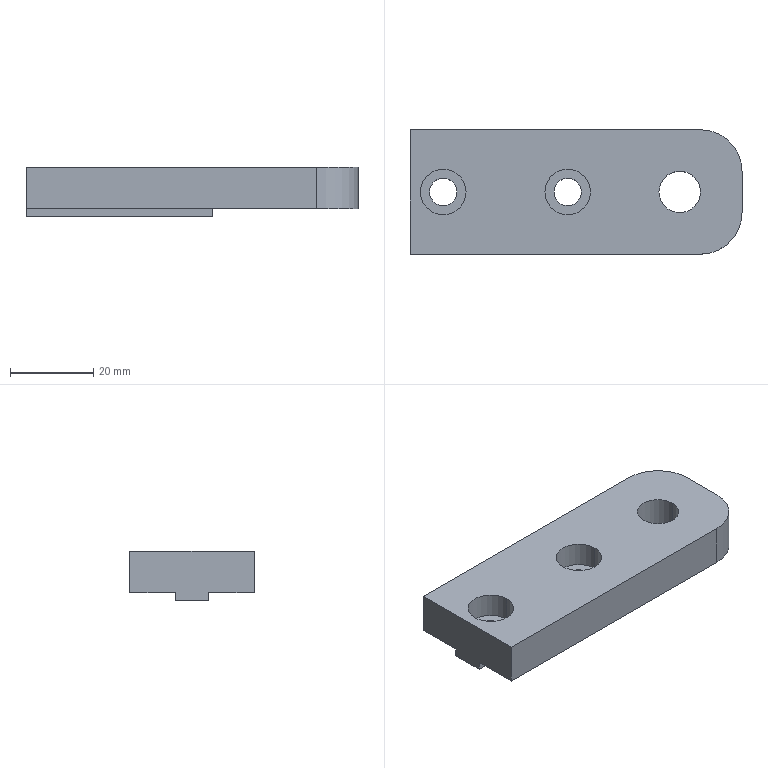Part | STEP file | 11-XSS10811 | 1 solid | 24 faces | box 80 x 30 x 12 mm | volume 21954 mm3 | cylinder 12 | plane 12 | commonest cylinder face diameters 6.6 x4 11 x4 10 x2 20 x2
STEP:
#1=CARTESIAN_POINT('',(-7.5,0.,4.));
#2=VERTEX_POINT('',#1);
#3=CARTESIAN_POINT('',(3.5,0.,4.));
#4=VERTEX_POINT('',#3);
#5=CARTESIAN_POINT('',(-2.,0.,4.));
#6=DIRECTION('',(0.,0.,1.));
#7=DIRECTION('',(1.,0.,0.));
#8=AXIS2_PLACEMENT_3D('',#5,#6,#7);
#9=CIRCLE('',#8,5.5);
#10=EDGE_CURVE('',#2,#4,#9,.T.);
#11=ORIENTED_EDGE('',*,*,#10,.F.);
#12=CARTESIAN_POINT('',(-7.5,0.,10.));
#13=VERTEX_POINT('',#12);
#14=CARTESIAN_POINT('',(-7.5,0.,10.));
#15=DIRECTION('',(0.,0.,1.));
#16=VECTOR('',#15,1000.);
#17=LINE('',#14,#16);
#18=EDGE_CURVE('',#2,#13,#17,.T.);
#19=ORIENTED_EDGE('',*,*,#18,.T.);
#20=CARTESIAN_POINT('',(3.5,0.,10.));
#21=VERTEX_POINT('',#20);
#22=CARTESIAN_POINT('',(-2.,0.,10.));
#23=DIRECTION('',(0.,0.,1.));
#24=DIRECTION('',(1.,0.,0.));
#25=AXIS2_PLACEMENT_3D('',#22,#23,#24);
#26=CIRCLE('',#25,5.5);
#27=EDGE_CURVE('',#13,#21,#26,.T.);
#28=ORIENTED_EDGE('',*,*,#27,.T.);
#29=CARTESIAN_POINT('',(3.5,0.,10.));
#30=DIRECTION('',(0.,0.,1.));
#31=VECTOR('',#30,1000.);
#32=LINE('',#29,#31);
#33=EDGE_CURVE('',#4,#21,#32,.T.);
#34=ORIENTED_EDGE('',*,*,#33,.F.);
#35=EDGE_LOOP('',(#11,#19,#28,#34));
#36=FACE_OUTER_BOUND('',#35,.T.);
#37=CARTESIAN_POINT('',(-2.,0.,10.));
#38=DIRECTION('',(0.,0.,1.));
#39=DIRECTION('',(1.,0.,0.));
#40=AXIS2_PLACEMENT_3D('',#37,#38,#39);
#41=CYLINDRICAL_SURFACE('',#40,5.5);
#42=ADVANCED_FACE('',(#36),#41,.F.);
#43=CARTESIAN_POINT('',(-5.3,0.,-2.));
#44=VERTEX_POINT('',#43);
#45=CARTESIAN_POINT('',(1.3,0.,-2.));
#46=VERTEX_POINT('',#45);
#47=CARTESIAN_POINT('',(-2.,0.,-2.));
#48=DIRECTION('',(0.,0.,1.));
#49=DIRECTION('',(1.,0.,0.));
#50=AXIS2_PLACEMENT_3D('',#47,#48,#49);
#51=CIRCLE('',#50,3.3);
#52=EDGE_CURVE('',#44,#46,#51,.T.);
#53=ORIENTED_EDGE('',*,*,#52,.F.);
#54=CARTESIAN_POINT('',(-5.3,0.,4.));
#55=VERTEX_POINT('',#54);
#56=CARTESIAN_POINT('',(-5.3,0.,10.));
#57=DIRECTION('',(0.,0.,1.));
#58=VECTOR('',#57,1000.);
#59=LINE('',#56,#58);
#60=EDGE_CURVE('',#44,#55,#59,.T.);
#61=ORIENTED_EDGE('',*,*,#60,.T.);
#62=CARTESIAN_POINT('',(1.3,0.,4.));
#63=VERTEX_POINT('',#62);
#64=CARTESIAN_POINT('',(-2.,0.,4.));
#65=DIRECTION('',(0.,0.,1.));
#66=DIRECTION('',(1.,0.,0.));
#67=AXIS2_PLACEMENT_3D('',#64,#65,#66);
#68=CIRCLE('',#67,3.3);
#69=EDGE_CURVE('',#55,#63,#68,.T.);
#70=ORIENTED_EDGE('',*,*,#69,.T.);
#71=CARTESIAN_POINT('',(1.3,0.,10.));
#72=DIRECTION('',(0.,0.,1.));
#73=VECTOR('',#72,1000.);
#74=LINE('',#71,#73);
#75=EDGE_CURVE('',#46,#63,#74,.T.);
#76=ORIENTED_EDGE('',*,*,#75,.F.);
#77=EDGE_LOOP('',(#53,#61,#70,#76));
#78=FACE_OUTER_BOUND('',#77,.T.);
#79=CARTESIAN_POINT('',(-2.,0.,10.));
#80=DIRECTION('',(0.,0.,1.));
#81=DIRECTION('',(1.,0.,0.));
#82=AXIS2_PLACEMENT_3D('',#79,#80,#81);
#83=CYLINDRICAL_SURFACE('',#82,3.3);
#84=ADVANCED_FACE('',(#78),#83,.F.);
#85=CARTESIAN_POINT('',(-37.5,0.,4.));
#86=VERTEX_POINT('',#85);
#87=CARTESIAN_POINT('',(-26.5,0.,4.));
#88=VERTEX_POINT('',#87);
#89=CARTESIAN_POINT('',(-32.,0.,4.));
#90=DIRECTION('',(0.,0.,1.));
#91=DIRECTION('',(1.,0.,0.));
#92=AXIS2_PLACEMENT_3D('',#89,#90,#91);
#93=CIRCLE('',#92,5.5);
#94=EDGE_CURVE('',#86,#88,#93,.T.);
#95=ORIENTED_EDGE('',*,*,#94,.F.);
#96=CARTESIAN_POINT('',(-37.5,0.,10.));
#97=VERTEX_POINT('',#96);
#98=CARTESIAN_POINT('',(-37.5,0.,10.));
#99=DIRECTION('',(0.,0.,1.));
#100=VECTOR('',#99,1000.);
#101=LINE('',#98,#100);
#102=EDGE_CURVE('',#86,#97,#101,.T.);
#103=ORIENTED_EDGE('',*,*,#102,.T.);
#104=CARTESIAN_POINT('',(-26.5,0.,10.));
#105=VERTEX_POINT('',#104);
#106=CARTESIAN_POINT('',(-32.,0.,10.));
#107=DIRECTION('',(0.,0.,1.));
#108=DIRECTION('',(1.,0.,0.));
#109=AXIS2_PLACEMENT_3D('',#106,#107,#108);
#110=CIRCLE('',#109,5.5);
#111=EDGE_CURVE('',#97,#105,#110,.T.);
#112=ORIENTED_EDGE('',*,*,#111,.T.);
#113=CARTESIAN_POINT('',(-26.5,0.,10.));
#114=DIRECTION('',(0.,0.,1.));
#115=VECTOR('',#114,1000.);
#116=LINE('',#113,#115);
#117=EDGE_CURVE('',#88,#105,#116,.T.);
#118=ORIENTED_EDGE('',*,*,#117,.F.);
#119=EDGE_LOOP('',(#95,#103,#112,#118));
#120=FACE_OUTER_BOUND('',#119,.T.);
#121=CARTESIAN_POINT('',(-32.,0.,10.));
#122=DIRECTION('',(0.,0.,1.));
#123=DIRECTION('',(1.,0.,0.));
#124=AXIS2_PLACEMENT_3D('',#121,#122,#123);
#125=CYLINDRICAL_SURFACE('',#124,5.5);
#126=ADVANCED_FACE('',(#120),#125,.F.);
#127=CARTESIAN_POINT('',(-35.3,0.,-2.));
#128=VERTEX_POINT('',#127);
#129=CARTESIAN_POINT('',(-28.7,0.,-2.));
#130=VERTEX_POINT('',#129);
#131=CARTESIAN_POINT('',(-32.,0.,-2.));
#132=DIRECTION('',(0.,0.,1.));
#133=DIRECTION('',(1.,0.,0.));
#134=AXIS2_PLACEMENT_3D('',#131,#132,#133);
#135=CIRCLE('',#134,3.3);
#136=EDGE_CURVE('',#128,#130,#135,.T.);
#137=ORIENTED_EDGE('',*,*,#136,.F.);
#138=CARTESIAN_POINT('',(-35.3,0.,4.));
#139=VERTEX_POINT('',#138);
#140=CARTESIAN_POINT('',(-35.3,0.,10.));
#141=DIRECTION('',(0.,0.,1.));
#142=VECTOR('',#141,1000.);
#143=LINE('',#140,#142);
#144=EDGE_CURVE('',#128,#139,#143,.T.);
#145=ORIENTED_EDGE('',*,*,#144,.T.);
#146=CARTESIAN_POINT('',(-28.7,0.,4.));
#147=VERTEX_POINT('',#146);
#148=CARTESIAN_POINT('',(-32.,0.,4.));
#149=DIRECTION('',(0.,0.,1.));
#150=DIRECTION('',(1.,0.,0.));
#151=AXIS2_PLACEMENT_3D('',#148,#149,#150);
#152=CIRCLE('',#151,3.3);
#153=EDGE_CURVE('',#139,#147,#152,.T.);
#154=ORIENTED_EDGE('',*,*,#153,.T.);
#155=CARTESIAN_POINT('',(-28.7,0.,10.));
#156=DIRECTION('',(0.,0.,1.));
#157=VECTOR('',#156,1000.);
#158=LINE('',#155,#157);
#159=EDGE_CURVE('',#130,#147,#158,.T.);
#160=ORIENTED_EDGE('',*,*,#159,.F.);
#161=EDGE_LOOP('',(#137,#145,#154,#160));
#162=FACE_OUTER_BOUND('',#161,.T.);
#163=CARTESIAN_POINT('',(-32.,0.,10.));
#164=DIRECTION('',(0.,0.,1.));
#165=DIRECTION('',(1.,0.,0.));
#166=AXIS2_PLACEMENT_3D('',#163,#164,#165);
#167=CYLINDRICAL_SURFACE('',#166,3.3);
#168=ADVANCED_FACE('',(#162),#167,.F.);
#169=CARTESIAN_POINT('',(20.,0.,0.));
#170=VERTEX_POINT('',#169);
#171=CARTESIAN_POINT('',(30.,0.,0.));
#172=VERTEX_POINT('',#171);
#173=CARTESIAN_POINT('',(25.,0.,0.));
#174=DIRECTION('',(0.,0.,1.));
#175=DIRECTION('',(1.,0.,0.));
#176=AXIS2_PLACEMENT_3D('',#173,#174,#175);
#177=CIRCLE('',#176,5.);
#178=EDGE_CURVE('',#170,#172,#177,.T.);
#179=ORIENTED_EDGE('',*,*,#178,.F.);
#180=CARTESIAN_POINT('',(20.,0.,10.));
#181=VERTEX_POINT('',#180);
#182=CARTESIAN_POINT('',(20.,0.,0.));
#183=DIRECTION('',(0.,0.,1.));
#184=VECTOR('',#183,1000.);
#185=LINE('',#182,#184);
#186=EDGE_CURVE('',#170,#181,#185,.T.);
#187=ORIENTED_EDGE('',*,*,#186,.T.);
#188=CARTESIAN_POINT('',(30.,0.,10.));
#189=VERTEX_POINT('',#188);
#190=CARTESIAN_POINT('',(25.,0.,10.));
#191=DIRECTION('',(0.,0.,1.));
#192=DIRECTION('',(1.,0.,0.));
#193=AXIS2_PLACEMENT_3D('',#190,#191,#192);
#194=CIRCLE('',#193,5.);
#195=EDGE_CURVE('',#181,#189,#194,.T.);
#196=ORIENTED_EDGE('',*,*,#195,.T.);
#197=CARTESIAN_POINT('',(30.,0.,0.));
#198=DIRECTION('',(0.,0.,1.));
#199=VECTOR('',#198,1000.);
#200=LINE('',#197,#199);
#201=EDGE_CURVE('',#172,#189,#200,.T.);
#202=ORIENTED_EDGE('',*,*,#201,.F.);
#203=EDGE_LOOP('',(#179,#187,#196,#202));
#204=FACE_OUTER_BOUND('',#203,.T.);
#205=CARTESIAN_POINT('',(25.,0.,0.));
#206=DIRECTION('',(0.,0.,1.));
#207=DIRECTION('',(1.,0.,0.));
#208=AXIS2_PLACEMENT_3D('',#205,#206,#207);
#209=CYLINDRICAL_SURFACE('',#208,5.);
#210=ADVANCED_FACE('',(#204),#209,.F.);
#211=CARTESIAN_POINT('',(25.,0.,0.));
#212=DIRECTION('',(0.,0.,1.));
#213=DIRECTION('',(1.,0.,0.));
#214=AXIS2_PLACEMENT_3D('',#211,#212,#213);
#215=CIRCLE('',#214,5.);
#216=EDGE_CURVE('',#172,#170,#215,.T.);
#217=ORIENTED_EDGE('',*,*,#216,.T.);
#218=ORIENTED_EDGE('',*,*,#178,.T.);
#219=EDGE_LOOP('',(#217,#218));
#220=FACE_BOUND('',#219,.T.);
#221=CARTESIAN_POINT('',(5.,-4.,0.));
#222=VERTEX_POINT('',#221);
#223=CARTESIAN_POINT('',(-40.,-4.,0.));
#224=VERTEX_POINT('',#223);
#225=CARTESIAN_POINT('',(-40.,-4.,0.));
#226=DIRECTION('',(-1.,0.,0.));
#227=VECTOR('',#226,1000.);
#228=LINE('',#225,#227);
#229=EDGE_CURVE('',#222,#224,#228,.T.);
#230=ORIENTED_EDGE('',*,*,#229,.F.);
#231=CARTESIAN_POINT('',(5.,4.,0.));
#232=VERTEX_POINT('',#231);
#233=CARTESIAN_POINT('',(5.,4.,0.));
#234=DIRECTION('',(0.,-1.,0.));
#235=VECTOR('',#234,1000.);
#236=LINE('',#233,#235);
#237=EDGE_CURVE('',#232,#222,#236,.T.);
#238=ORIENTED_EDGE('',*,*,#237,.F.);
#239=CARTESIAN_POINT('',(-40.,4.,0.));
#240=VERTEX_POINT('',#239);
#241=CARTESIAN_POINT('',(-40.,4.,0.));
#242=DIRECTION('',(1.,0.,0.));
#243=VECTOR('',#242,1000.);
#244=LINE('',#241,#243);
#245=EDGE_CURVE('',#240,#232,#244,.T.);
#246=ORIENTED_EDGE('',*,*,#245,.F.);
#247=CARTESIAN_POINT('',(-40.,15.,0.));
#248=VERTEX_POINT('',#247);
#249=CARTESIAN_POINT('',(-40.,15.,0.));
#250=DIRECTION('',(0.,-1.,0.));
#251=VECTOR('',#250,1000.);
#252=LINE('',#249,#251);
#253=EDGE_CURVE('',#248,#240,#252,.T.);
#254=ORIENTED_EDGE('',*,*,#253,.F.);
#255=CARTESIAN_POINT('',(30.,15.,0.));
#256=VERTEX_POINT('',#255);
#257=CARTESIAN_POINT('',(-40.,15.,0.));
#258=DIRECTION('',(-1.,0.,0.));
#259=VECTOR('',#258,1000.);
#260=LINE('',#257,#259);
#261=EDGE_CURVE('',#256,#248,#260,.T.);
#262=ORIENTED_EDGE('',*,*,#261,.F.);
#263=CARTESIAN_POINT('',(40.,5.,0.));
#264=VERTEX_POINT('',#263);
#265=CARTESIAN_POINT('',(30.,5.,0.));
#266=DIRECTION('',(0.,0.,-1.));
#267=DIRECTION('',(1.,0.,0.));
#268=AXIS2_PLACEMENT_3D('',#265,#266,#267);
#269=CIRCLE('',#268,10.);
#270=EDGE_CURVE('',#256,#264,#269,.T.);
#271=ORIENTED_EDGE('',*,*,#270,.T.);
#272=CARTESIAN_POINT('',(40.,-5.,0.));
#273=VERTEX_POINT('',#272);
#274=CARTESIAN_POINT('',(40.,15.,0.));
#275=DIRECTION('',(0.,1.,0.));
#276=VECTOR('',#275,1000.);
#277=LINE('',#274,#276);
#278=EDGE_CURVE('',#273,#264,#277,.T.);
#279=ORIENTED_EDGE('',*,*,#278,.F.);
#280=CARTESIAN_POINT('',(30.,-15.,0.));
#281=VERTEX_POINT('',#280);
#282=CARTESIAN_POINT('',(30.,-5.,0.));
#283=DIRECTION('',(0.,0.,-1.));
#284=DIRECTION('',(1.,0.,0.));
#285=AXIS2_PLACEMENT_3D('',#282,#283,#284);
#286=CIRCLE('',#285,10.);
#287=EDGE_CURVE('',#273,#281,#286,.T.);
#288=ORIENTED_EDGE('',*,*,#287,.T.);
#289=CARTESIAN_POINT('',(-40.,-15.,0.));
#290=VERTEX_POINT('',#289);
#291=CARTESIAN_POINT('',(-40.,-15.,0.));
#292=DIRECTION('',(1.,0.,0.));
#293=VECTOR('',#292,1000.);
#294=LINE('',#291,#293);
#295=EDGE_CURVE('',#290,#281,#294,.T.);
#296=ORIENTED_EDGE('',*,*,#295,.F.);
#297=CARTESIAN_POINT('',(-40.,15.,0.));
#298=DIRECTION('',(0.,-1.,0.));
#299=VECTOR('',#298,1000.);
#300=LINE('',#297,#299);
#301=EDGE_CURVE('',#224,#290,#300,.T.);
#302=ORIENTED_EDGE('',*,*,#301,.F.);
#303=EDGE_LOOP('',(#230,#238,#246,#254,#262,#271,#279,#288,#296,#302));
#304=FACE_OUTER_BOUND('',#303,.T.);
#305=CARTESIAN_POINT('',(40.,-15.,0.));
#306=DIRECTION('',(0.,0.,1.));
#307=DIRECTION('',(1.,0.,0.));
#308=AXIS2_PLACEMENT_3D('',#305,#306,#307);
#309=PLANE('',#308);
#310=ADVANCED_FACE('',(#220,#304),#309,.F.);
#311=CARTESIAN_POINT('',(40.,-5.,10.));
#312=VERTEX_POINT('',#311);
#313=CARTESIAN_POINT('',(40.,5.,10.));
#314=VERTEX_POINT('',#313);
#315=CARTESIAN_POINT('',(40.,15.,10.));
#316=DIRECTION('',(0.,1.,0.));
#317=VECTOR('',#316,1000.);
#318=LINE('',#315,#317);
#319=EDGE_CURVE('',#312,#314,#318,.T.);
#320=ORIENTED_EDGE('',*,*,#319,.F.);
#321=CARTESIAN_POINT('',(40.,-5.,10.));
#322=DIRECTION('',(0.,0.,-1.));
#323=VECTOR('',#322,1000.);
#324=LINE('',#321,#323);
#325=EDGE_CURVE('',#312,#273,#324,.T.);
#326=ORIENTED_EDGE('',*,*,#325,.T.);
#327=ORIENTED_EDGE('',*,*,#278,.T.);
#328=CARTESIAN_POINT('',(40.,5.,10.));
#329=DIRECTION('',(0.,0.,1.));
#330=VECTOR('',#329,1000.);
#331=LINE('',#328,#330);
#332=EDGE_CURVE('',#264,#314,#331,.T.);
#333=ORIENTED_EDGE('',*,*,#332,.T.);
#334=EDGE_LOOP('',(#320,#326,#327,#333));
#335=FACE_OUTER_BOUND('',#334,.T.);
#336=CARTESIAN_POINT('',(40.,15.,10.));
#337=DIRECTION('',(-1.,0.,0.));
#338=DIRECTION('',(0.,-1.,0.));
#339=AXIS2_PLACEMENT_3D('',#336,#337,#338);
#340=PLANE('',#339);
#341=ADVANCED_FACE('',(#335),#340,.F.);
#342=CARTESIAN_POINT('',(30.,15.,10.));
#343=VERTEX_POINT('',#342);
#344=CARTESIAN_POINT('',(-40.,15.,10.));
#345=VERTEX_POINT('',#344);
#346=CARTESIAN_POINT('',(-40.,15.,10.));
#347=DIRECTION('',(-1.,0.,0.));
#348=VECTOR('',#347,1000.);
#349=LINE('',#346,#348);
#350=EDGE_CURVE('',#343,#345,#349,.T.);
#351=ORIENTED_EDGE('',*,*,#350,.F.);
#352=CARTESIAN_POINT('',(30.,15.,10.));
#353=DIRECTION('',(0.,0.,-1.));
#354=VECTOR('',#353,1000.);
#355=LINE('',#352,#354);
#356=EDGE_CURVE('',#343,#256,#355,.T.);
#357=ORIENTED_EDGE('',*,*,#356,.T.);
#358=ORIENTED_EDGE('',*,*,#261,.T.);
#359=CARTESIAN_POINT('',(-40.,15.,10.));
#360=DIRECTION('',(0.,0.,-1.));
#361=VECTOR('',#360,1000.);
#362=LINE('',#359,#361);
#363=EDGE_CURVE('',#345,#248,#362,.T.);
#364=ORIENTED_EDGE('',*,*,#363,.F.);
#365=EDGE_LOOP('',(#351,#357,#358,#364));
#366=FACE_OUTER_BOUND('',#365,.T.);
#367=CARTESIAN_POINT('',(-40.,15.,10.));
#368=DIRECTION('',(0.,-1.,0.));
#369=DIRECTION('',(0.,0.,-1.));
#370=AXIS2_PLACEMENT_3D('',#367,#368,#369);
#371=PLANE('',#370);
#372=ADVANCED_FACE('',(#366),#371,.F.);
#373=ORIENTED_EDGE('',*,*,#253,.T.);
#374=CARTESIAN_POINT('',(-40.,4.,-2.));
#375=VERTEX_POINT('',#374);
#376=CARTESIAN_POINT('',(-40.,4.,-2.));
#377=DIRECTION('',(0.,0.,1.));
#378=VECTOR('',#377,1000.);
#379=LINE('',#376,#378);
#380=EDGE_CURVE('',#375,#240,#379,.T.);
#381=ORIENTED_EDGE('',*,*,#380,.F.);
#382=CARTESIAN_POINT('',(-40.,-4.,-2.));
#383=VERTEX_POINT('',#382);
#384=CARTESIAN_POINT('',(-40.,4.,-2.));
#385=DIRECTION('',(0.,1.,0.));
#386=VECTOR('',#385,1000.);
#387=LINE('',#384,#386);
#388=EDGE_CURVE('',#383,#375,#387,.T.);
#389=ORIENTED_EDGE('',*,*,#388,.F.);
#390=CARTESIAN_POINT('',(-40.,-4.,-2.));
#391=DIRECTION('',(0.,0.,1.));
#392=VECTOR('',#391,1000.);
#393=LINE('',#390,#392);
#394=EDGE_CURVE('',#383,#224,#393,.T.);
#395=ORIENTED_EDGE('',*,*,#394,.T.);
#396=ORIENTED_EDGE('',*,*,#301,.T.);
#397=CARTESIAN_POINT('',(-40.,-15.,10.));
#398=VERTEX_POINT('',#397);
#399=CARTESIAN_POINT('',(-40.,-15.,10.));
#400=DIRECTION('',(0.,0.,-1.));
#401=VECTOR('',#400,1000.);
#402=LINE('',#399,#401);
#403=EDGE_CURVE('',#398,#290,#402,.T.);
#404=ORIENTED_EDGE('',*,*,#403,.F.);
#405=CARTESIAN_POINT('',(-40.,15.,10.));
#406=DIRECTION('',(0.,-1.,0.));
#407=VECTOR('',#406,1000.);
#408=LINE('',#405,#407);
#409=EDGE_CURVE('',#345,#398,#408,.T.);
#410=ORIENTED_EDGE('',*,*,#409,.F.);
#411=ORIENTED_EDGE('',*,*,#363,.T.);
#412=EDGE_LOOP('',(#373,#381,#389,#395,#396,#404,#410,#411));
#413=FACE_OUTER_BOUND('',#412,.T.);
#414=CARTESIAN_POINT('',(-40.,15.,10.));
#415=DIRECTION('',(1.,0.,0.));
#416=DIRECTION('',(0.,1.,0.));
#417=AXIS2_PLACEMENT_3D('',#414,#415,#416);
#418=PLANE('',#417);
#419=ADVANCED_FACE('',(#413),#418,.F.);
#420=ORIENTED_EDGE('',*,*,#295,.T.);
#421=CARTESIAN_POINT('',(30.,-15.,10.));
#422=VERTEX_POINT('',#421);
#423=CARTESIAN_POINT('',(30.,-15.,10.));
#424=DIRECTION('',(0.,0.,1.));
#425=VECTOR('',#424,1000.);
#426=LINE('',#423,#425);
#427=EDGE_CURVE('',#281,#422,#426,.T.);
#428=ORIENTED_EDGE('',*,*,#427,.T.);
#429=CARTESIAN_POINT('',(-40.,-15.,10.));
#430=DIRECTION('',(1.,0.,0.));
#431=VECTOR('',#430,1000.);
#432=LINE('',#429,#431);
#433=EDGE_CURVE('',#398,#422,#432,.T.);
#434=ORIENTED_EDGE('',*,*,#433,.F.);
#435=ORIENTED_EDGE('',*,*,#403,.T.);
#436=EDGE_LOOP('',(#420,#428,#434,#435));
#437=FACE_OUTER_BOUND('',#436,.T.);
#438=CARTESIAN_POINT('',(-40.,-15.,10.));
#439=DIRECTION('',(0.,1.,0.));
#440=DIRECTION('',(0.,0.,1.));
#441=AXIS2_PLACEMENT_3D('',#438,#439,#440);
#442=PLANE('',#441);
#443=ADVANCED_FACE('',(#437),#442,.F.);
#444=CARTESIAN_POINT('',(-2.,0.,10.));
#445=DIRECTION('',(0.,0.,1.));
#446=DIRECTION('',(1.,0.,0.));
#447=AXIS2_PLACEMENT_3D('',#444,#445,#446);
#448=CIRCLE('',#447,5.5);
#449=EDGE_CURVE('',#21,#13,#448,.T.);
#450=ORIENTED_EDGE('',*,*,#449,.F.);
#451=ORIENTED_EDGE('',*,*,#27,.F.);
#452=EDGE_LOOP('',(#450,#451));
#453=FACE_BOUND('',#452,.T.);
#454=CARTESIAN_POINT('',(-32.,0.,10.));
#455=DIRECTION('',(0.,0.,1.));
#456=DIRECTION('',(1.,0.,0.));
#457=AXIS2_PLACEMENT_3D('',#454,#455,#456);
#458=CIRCLE('',#457,5.5);
#459=EDGE_CURVE('',#105,#97,#458,.T.);
#460=ORIENTED_EDGE('',*,*,#459,.F.);
#461=ORIENTED_EDGE('',*,*,#111,.F.);
#462=EDGE_LOOP('',(#460,#461));
#463=FACE_BOUND('',#462,.T.);
#464=CARTESIAN_POINT('',(25.,0.,10.));
#465=DIRECTION('',(0.,0.,1.));
#466=DIRECTION('',(1.,0.,0.));
#467=AXIS2_PLACEMENT_3D('',#464,#465,#466);
#468=CIRCLE('',#467,5.);
#469=EDGE_CURVE('',#189,#181,#468,.T.);
#470=ORIENTED_EDGE('',*,*,#469,.F.);
#471=ORIENTED_EDGE('',*,*,#195,.F.);
#472=EDGE_LOOP('',(#470,#471));
#473=FACE_BOUND('',#472,.T.);
#474=ORIENTED_EDGE('',*,*,#433,.T.);
#475=CARTESIAN_POINT('',(30.,-5.,10.));
#476=DIRECTION('',(0.,0.,1.));
#477=DIRECTION('',(1.,0.,0.));
#478=AXIS2_PLACEMENT_3D('',#475,#476,#477);
#479=CIRCLE('',#478,10.);
#480=EDGE_CURVE('',#422,#312,#479,.T.);
#481=ORIENTED_EDGE('',*,*,#480,.T.);
#482=ORIENTED_EDGE('',*,*,#319,.T.);
#483=CARTESIAN_POINT('',(30.,5.,10.));
#484=DIRECTION('',(0.,0.,1.));
#485=DIRECTION('',(1.,0.,0.));
#486=AXIS2_PLACEMENT_3D('',#483,#484,#485);
#487=CIRCLE('',#486,10.);
#488=EDGE_CURVE('',#314,#343,#487,.T.);
#489=ORIENTED_EDGE('',*,*,#488,.T.);
#490=ORIENTED_EDGE('',*,*,#350,.T.);
#491=ORIENTED_EDGE('',*,*,#409,.T.);
#492=EDGE_LOOP('',(#474,#481,#482,#489,#490,#491));
#493=FACE_OUTER_BOUND('',#492,.T.);
#494=CARTESIAN_POINT('',(40.,-15.,10.));
#495=DIRECTION('',(0.,0.,1.));
#496=DIRECTION('',(1.,0.,0.));
#497=AXIS2_PLACEMENT_3D('',#494,#495,#496);
#498=PLANE('',#497);
#499=ADVANCED_FACE('',(#453,#463,#473,#493),#498,.T.);
#500=ORIENTED_EDGE('',*,*,#186,.F.);
#501=ORIENTED_EDGE('',*,*,#216,.F.);
#502=ORIENTED_EDGE('',*,*,#201,.T.);
#503=ORIENTED_EDGE('',*,*,#469,.T.);
#504=EDGE_LOOP('',(#500,#501,#502,#503));
#505=FACE_OUTER_BOUND('',#504,.T.);
#506=CARTESIAN_POINT('',(25.,0.,0.));
#507=DIRECTION('',(0.,0.,1.));
#508=DIRECTION('',(1.,0.,0.));
#509=AXIS2_PLACEMENT_3D('',#506,#507,#508);
#510=CYLINDRICAL_SURFACE('',#509,5.);
#511=ADVANCED_FACE('',(#505),#510,.F.);
#512=ORIENTED_EDGE('',*,*,#480,.F.);
#513=ORIENTED_EDGE('',*,*,#427,.F.);
#514=ORIENTED_EDGE('',*,*,#287,.F.);
#515=ORIENTED_EDGE('',*,*,#325,.F.);
#516=EDGE_LOOP('',(#512,#513,#514,#515));
#517=FACE_OUTER_BOUND('',#516,.T.);
#518=CARTESIAN_POINT('',(30.,-5.,10.));
#519=DIRECTION('',(0.,0.,-1.));
#520=DIRECTION('',(-1.,0.,0.));
#521=AXIS2_PLACEMENT_3D('',#518,#519,#520);
#522=CYLINDRICAL_SURFACE('',#521,10.);
#523=ADVANCED_FACE('',(#517),#522,.T.);
#524=ORIENTED_EDGE('',*,*,#488,.F.);
#525=ORIENTED_EDGE('',*,*,#332,.F.);
#526=ORIENTED_EDGE('',*,*,#270,.F.);
#527=ORIENTED_EDGE('',*,*,#356,.F.);
#528=EDGE_LOOP('',(#524,#525,#526,#527));
#529=FACE_OUTER_BOUND('',#528,.T.);
#530=CARTESIAN_POINT('',(30.,5.,10.));
#531=DIRECTION('',(0.,0.,-1.));
#532=DIRECTION('',(-1.,0.,0.));
#533=AXIS2_PLACEMENT_3D('',#530,#531,#532);
#534=CYLINDRICAL_SURFACE('',#533,10.);
#535=ADVANCED_FACE('',(#529),#534,.T.);
#536=ORIENTED_EDGE('',*,*,#245,.T.);
#537=CARTESIAN_POINT('',(5.,4.,-2.));
#538=VERTEX_POINT('',#537);
#539=CARTESIAN_POINT('',(5.,4.,-2.));
#540=DIRECTION('',(0.,0.,1.));
#541=VECTOR('',#540,1000.);
#542=LINE('',#539,#541);
#543=EDGE_CURVE('',#538,#232,#542,.T.);
#544=ORIENTED_EDGE('',*,*,#543,.F.);
#545=CARTESIAN_POINT('',(-40.,4.,-2.));
#546=DIRECTION('',(1.,0.,0.));
#547=VECTOR('',#546,1000.);
#548=LINE('',#545,#547);
#549=EDGE_CURVE('',#375,#538,#548,.T.);
#550=ORIENTED_EDGE('',*,*,#549,.F.);
#551=ORIENTED_EDGE('',*,*,#380,.T.);
#552=EDGE_LOOP('',(#536,#544,#550,#551));
#553=FACE_OUTER_BOUND('',#552,.T.);
#554=CARTESIAN_POINT('',(-40.,4.,-2.));
#555=DIRECTION('',(0.,-1.,0.));
#556=DIRECTION('',(1.,0.,0.));
#557=AXIS2_PLACEMENT_3D('',#554,#555,#556);
#558=PLANE('',#557);
#559=ADVANCED_FACE('',(#553),#558,.F.);
#560=ORIENTED_EDGE('',*,*,#237,.T.);
#561=CARTESIAN_POINT('',(5.,-4.,-2.));
#562=VERTEX_POINT('',#561);
#563=CARTESIAN_POINT('',(5.,-4.,-2.));
#564=DIRECTION('',(0.,0.,1.));
#565=VECTOR('',#564,1000.);
#566=LINE('',#563,#565);
#567=EDGE_CURVE('',#562,#222,#566,.T.);
#568=ORIENTED_EDGE('',*,*,#567,.F.);
#569=CARTESIAN_POINT('',(5.,4.,-2.));
#570=DIRECTION('',(0.,-1.,0.));
#571=VECTOR('',#570,1000.);
#572=LINE('',#569,#571);
#573=EDGE_CURVE('',#538,#562,#572,.T.);
#574=ORIENTED_EDGE('',*,*,#573,.F.);
#575=ORIENTED_EDGE('',*,*,#543,.T.);
#576=EDGE_LOOP('',(#560,#568,#574,#575));
#577=FACE_OUTER_BOUND('',#576,.T.);
#578=CARTESIAN_POINT('',(5.,4.,-2.));
#579=DIRECTION('',(-1.,0.,0.));
#580=DIRECTION('',(0.,0.,1.));
#581=AXIS2_PLACEMENT_3D('',#578,#579,#580);
#582=PLANE('',#581);
#583=ADVANCED_FACE('',(#577),#582,.F.);
#584=ORIENTED_EDGE('',*,*,#229,.T.);
#585=ORIENTED_EDGE('',*,*,#394,.F.);
#586=CARTESIAN_POINT('',(-40.,-4.,-2.));
#587=DIRECTION('',(-1.,0.,0.));
#588=VECTOR('',#587,1000.);
#589=LINE('',#586,#588);
#590=EDGE_CURVE('',#562,#383,#589,.T.);
#591=ORIENTED_EDGE('',*,*,#590,.F.);
#592=ORIENTED_EDGE('',*,*,#567,.T.);
#593=EDGE_LOOP('',(#584,#585,#591,#592));
#594=FACE_OUTER_BOUND('',#593,.T.);
#595=CARTESIAN_POINT('',(-40.,-4.,-2.));
#596=DIRECTION('',(0.,1.,0.));
#597=DIRECTION('',(-1.,0.,0.));
#598=AXIS2_PLACEMENT_3D('',#595,#596,#597);
#599=PLANE('',#598);
#600=ADVANCED_FACE('',(#594),#599,.F.);
#601=CARTESIAN_POINT('',(-2.,0.,-2.));
#602=DIRECTION('',(0.,0.,1.));
#603=DIRECTION('',(1.,0.,0.));
#604=AXIS2_PLACEMENT_3D('',#601,#602,#603);
#605=CIRCLE('',#604,3.3);
#606=EDGE_CURVE('',#46,#44,#605,.T.);
#607=ORIENTED_EDGE('',*,*,#606,.T.);
#608=ORIENTED_EDGE('',*,*,#52,.T.);
#609=EDGE_LOOP('',(#607,#608));
#610=FACE_BOUND('',#609,.T.);
#611=CARTESIAN_POINT('',(-32.,0.,-2.));
#612=DIRECTION('',(0.,0.,1.));
#613=DIRECTION('',(1.,0.,0.));
#614=AXIS2_PLACEMENT_3D('',#611,#612,#613);
#615=CIRCLE('',#614,3.3);
#616=EDGE_CURVE('',#130,#128,#615,.T.);
#617=ORIENTED_EDGE('',*,*,#616,.T.);
#618=ORIENTED_EDGE('',*,*,#136,.T.);
#619=EDGE_LOOP('',(#617,#618));
#620=FACE_BOUND('',#619,.T.);
#621=ORIENTED_EDGE('',*,*,#388,.T.);
#622=ORIENTED_EDGE('',*,*,#549,.T.);
#623=ORIENTED_EDGE('',*,*,#573,.T.);
#624=ORIENTED_EDGE('',*,*,#590,.T.);
#625=EDGE_LOOP('',(#621,#622,#623,#624));
#626=FACE_OUTER_BOUND('',#625,.T.);
#627=CARTESIAN_POINT('',(-40.,-4.,-2.));
#628=DIRECTION('',(0.,0.,1.));
#629=DIRECTION('',(1.,0.,0.));
#630=AXIS2_PLACEMENT_3D('',#627,#628,#629);
#631=PLANE('',#630);
#632=ADVANCED_FACE('',(#610,#620,#626),#631,.F.);
#633=ORIENTED_EDGE('',*,*,#144,.F.);
#634=ORIENTED_EDGE('',*,*,#616,.F.);
#635=ORIENTED_EDGE('',*,*,#159,.T.);
#636=CARTESIAN_POINT('',(-32.,0.,4.));
#637=DIRECTION('',(0.,0.,1.));
#638=DIRECTION('',(1.,0.,0.));
#639=AXIS2_PLACEMENT_3D('',#636,#637,#638);
#640=CIRCLE('',#639,3.3);
#641=EDGE_CURVE('',#147,#139,#640,.T.);
#642=ORIENTED_EDGE('',*,*,#641,.T.);
#643=EDGE_LOOP('',(#633,#634,#635,#642));
#644=FACE_OUTER_BOUND('',#643,.T.);
#645=CARTESIAN_POINT('',(-32.,0.,10.));
#646=DIRECTION('',(0.,0.,1.));
#647=DIRECTION('',(1.,0.,0.));
#648=AXIS2_PLACEMENT_3D('',#645,#646,#647);
#649=CYLINDRICAL_SURFACE('',#648,3.3);
#650=ADVANCED_FACE('',(#644),#649,.F.);
#651=ORIENTED_EDGE('',*,*,#641,.F.);
#652=ORIENTED_EDGE('',*,*,#153,.F.);
#653=EDGE_LOOP('',(#651,#652));
#654=FACE_BOUND('',#653,.T.);
#655=CARTESIAN_POINT('',(-32.,0.,4.));
#656=DIRECTION('',(0.,0.,1.));
#657=DIRECTION('',(1.,0.,0.));
#658=AXIS2_PLACEMENT_3D('',#655,#656,#657);
#659=CIRCLE('',#658,5.5);
#660=EDGE_CURVE('',#88,#86,#659,.T.);
#661=ORIENTED_EDGE('',*,*,#660,.T.);
#662=ORIENTED_EDGE('',*,*,#94,.T.);
#663=EDGE_LOOP('',(#661,#662));
#664=FACE_OUTER_BOUND('',#663,.T.);
#665=CARTESIAN_POINT('',(-28.7,0.,4.));
#666=DIRECTION('',(0.,0.,-1.));
#667=DIRECTION('',(-1.,0.,0.));
#668=AXIS2_PLACEMENT_3D('',#665,#666,#667);
#669=PLANE('',#668);
#670=ADVANCED_FACE('',(#654,#664),#669,.F.);
#671=ORIENTED_EDGE('',*,*,#102,.F.);
#672=ORIENTED_EDGE('',*,*,#660,.F.);
#673=ORIENTED_EDGE('',*,*,#117,.T.);
#674=ORIENTED_EDGE('',*,*,#459,.T.);
#675=EDGE_LOOP('',(#671,#672,#673,#674));
#676=FACE_OUTER_BOUND('',#675,.T.);
#677=CARTESIAN_POINT('',(-32.,0.,10.));
#678=DIRECTION('',(0.,0.,1.));
#679=DIRECTION('',(1.,0.,0.));
#680=AXIS2_PLACEMENT_3D('',#677,#678,#679);
#681=CYLINDRICAL_SURFACE('',#680,5.5);
#682=ADVANCED_FACE('',(#676),#681,.F.);
#683=ORIENTED_EDGE('',*,*,#60,.F.);
#684=ORIENTED_EDGE('',*,*,#606,.F.);
#685=ORIENTED_EDGE('',*,*,#75,.T.);
#686=CARTESIAN_POINT('',(-2.,0.,4.));
#687=DIRECTION('',(0.,0.,1.));
#688=DIRECTION('',(1.,0.,0.));
#689=AXIS2_PLACEMENT_3D('',#686,#687,#688);
#690=CIRCLE('',#689,3.3);
#691=EDGE_CURVE('',#63,#55,#690,.T.);
#692=ORIENTED_EDGE('',*,*,#691,.T.);
#693=EDGE_LOOP('',(#683,#684,#685,#692));
#694=FACE_OUTER_BOUND('',#693,.T.);
#695=CARTESIAN_POINT('',(-2.,0.,10.));
#696=DIRECTION('',(0.,0.,1.));
#697=DIRECTION('',(1.,0.,0.));
#698=AXIS2_PLACEMENT_3D('',#695,#696,#697);
#699=CYLINDRICAL_SURFACE('',#698,3.3);
#700=ADVANCED_FACE('',(#694),#699,.F.);
#701=ORIENTED_EDGE('',*,*,#691,.F.);
#702=ORIENTED_EDGE('',*,*,#69,.F.);
#703=EDGE_LOOP('',(#701,#702));
#704=FACE_BOUND('',#703,.T.);
#705=CARTESIAN_POINT('',(-2.,0.,4.));
#706=DIRECTION('',(0.,0.,1.));
#707=DIRECTION('',(1.,0.,0.));
#708=AXIS2_PLACEMENT_3D('',#705,#706,#707);
#709=CIRCLE('',#708,5.5);
#710=EDGE_CURVE('',#4,#2,#709,.T.);
#711=ORIENTED_EDGE('',*,*,#710,.T.);
#712=ORIENTED_EDGE('',*,*,#10,.T.);
#713=EDGE_LOOP('',(#711,#712));
#714=FACE_OUTER_BOUND('',#713,.T.);
#715=CARTESIAN_POINT('',(1.3,0.,4.));
#716=DIRECTION('',(0.,0.,-1.));
#717=DIRECTION('',(-1.,0.,0.));
#718=AXIS2_PLACEMENT_3D('',#715,#716,#717);
#719=PLANE('',#718);
#720=ADVANCED_FACE('',(#704,#714),#719,.F.);
#721=ORIENTED_EDGE('',*,*,#18,.F.);
#722=ORIENTED_EDGE('',*,*,#710,.F.);
#723=ORIENTED_EDGE('',*,*,#33,.T.);
#724=ORIENTED_EDGE('',*,*,#449,.T.);
#725=EDGE_LOOP('',(#721,#722,#723,#724));
#726=FACE_OUTER_BOUND('',#725,.T.);
#727=CARTESIAN_POINT('',(-2.,0.,10.));
#728=DIRECTION('',(0.,0.,1.));
#729=DIRECTION('',(1.,0.,0.));
#730=AXIS2_PLACEMENT_3D('',#727,#728,#729);
#731=CYLINDRICAL_SURFACE('',#730,5.5);
#732=ADVANCED_FACE('',(#726),#731,.F.);
#733=CLOSED_SHELL('',(#42,#84,#126,#168,#210,#310,#341,#372,#419,#443,#499,#511,#523,#535,#559,#583,#600,#632,#650,#670,#682,#700,#720,#732));
#734=MANIFOLD_SOLID_BREP('',#733);
#735=CARTESIAN_POINT('',(0.,0.,0.));
#736=DIRECTION('',(0.,0.,1.));
#737=DIRECTION('',(1.,0.,0.));
#738=AXIS2_PLACEMENT_3D('',#735,#736,#737);
#739=(LENGTH_UNIT()NAMED_UNIT(*)SI_UNIT(.MILLI.,.METRE.));
#740=UNCERTAINTY_MEASURE_WITH_UNIT(LENGTH_MEASURE(0.00001),#739,'','');
#741=(NAMED_UNIT(*)PLANE_ANGLE_UNIT()SI_UNIT($,.RADIAN.));
#742=(NAMED_UNIT(*)SI_UNIT($,.STERADIAN.)SOLID_ANGLE_UNIT());
#743=(GEOMETRIC_REPRESENTATION_CONTEXT(3)GLOBAL_UNCERTAINTY_ASSIGNED_CONTEXT((#740))GLOBAL_UNIT_ASSIGNED_CONTEXT((#739,#741,#742))REPRESENTATION_CONTEXT('',''));
#744=ADVANCED_BREP_SHAPE_REPRESENTATION('',(#734,#738),#743);